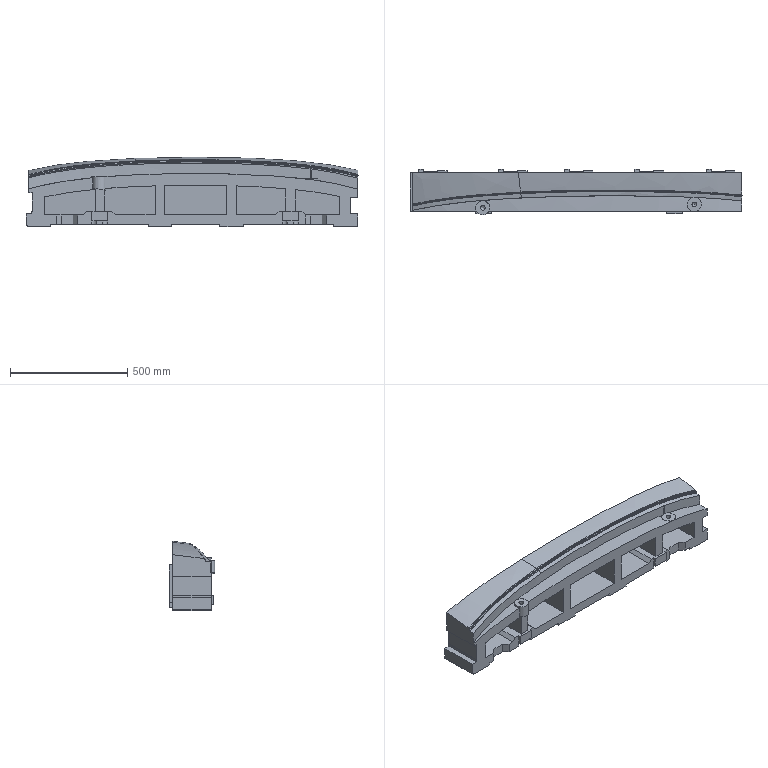Part | NX | features MAIN_BODY 2 | 1 solid | 185 faces | box 1413 x 195 x 295.73 mm | volume 41110805 mm3 | plane 124 | spline 43 | cylinder 16 | cone 2 | commonest cylinder face diameters 60 x6 32 x4 20 x2 3.001 x1 5.002 x1 5.004 x1